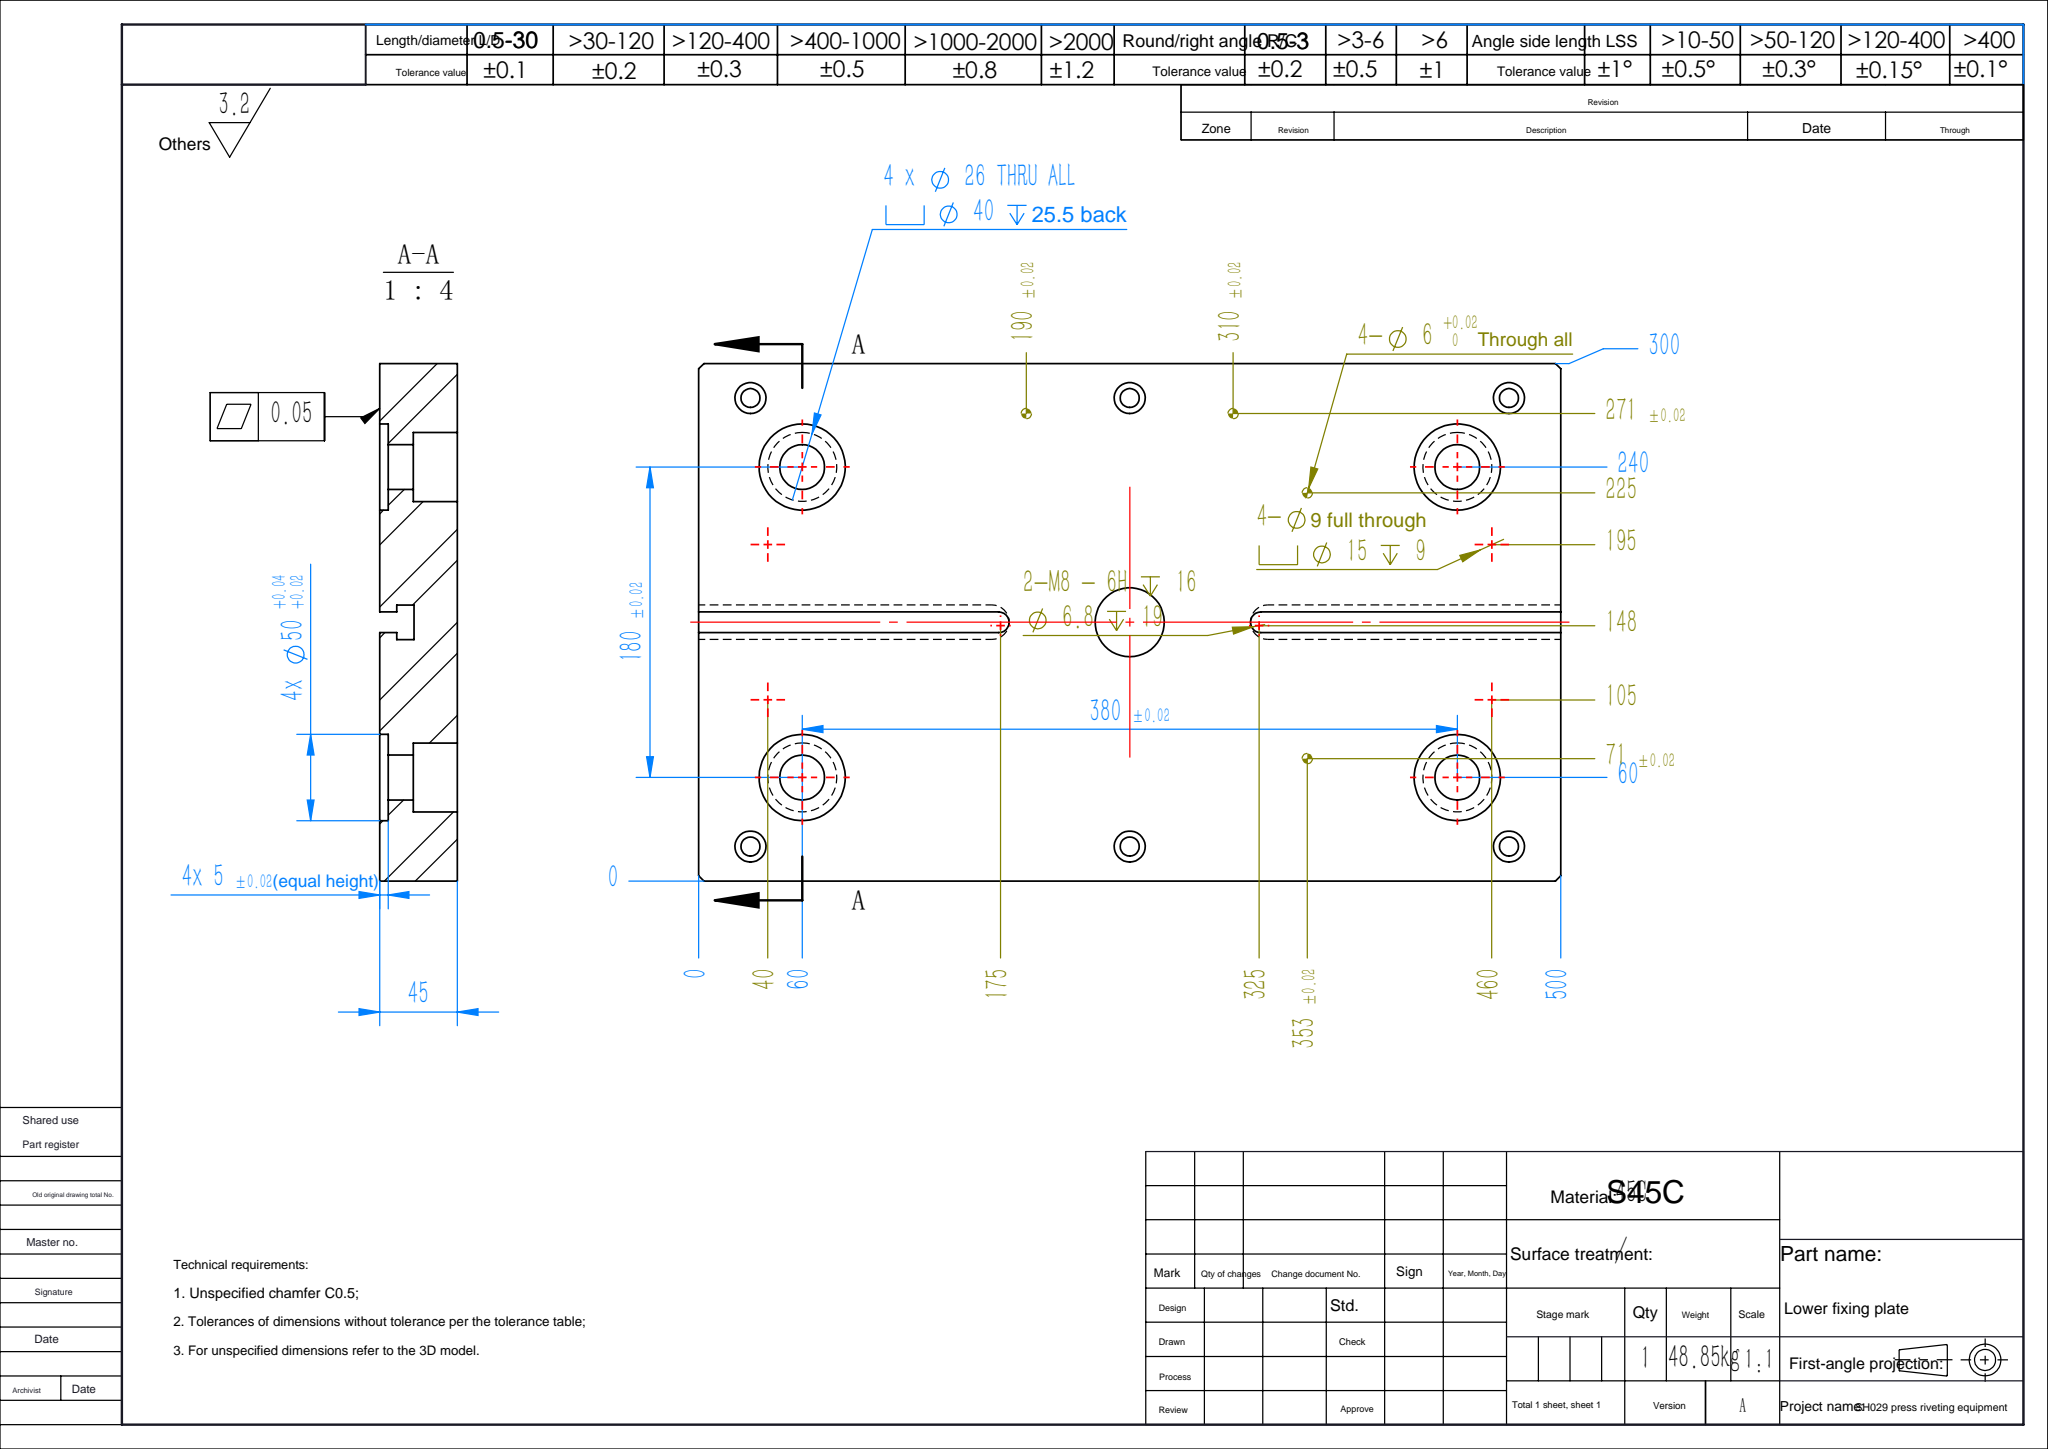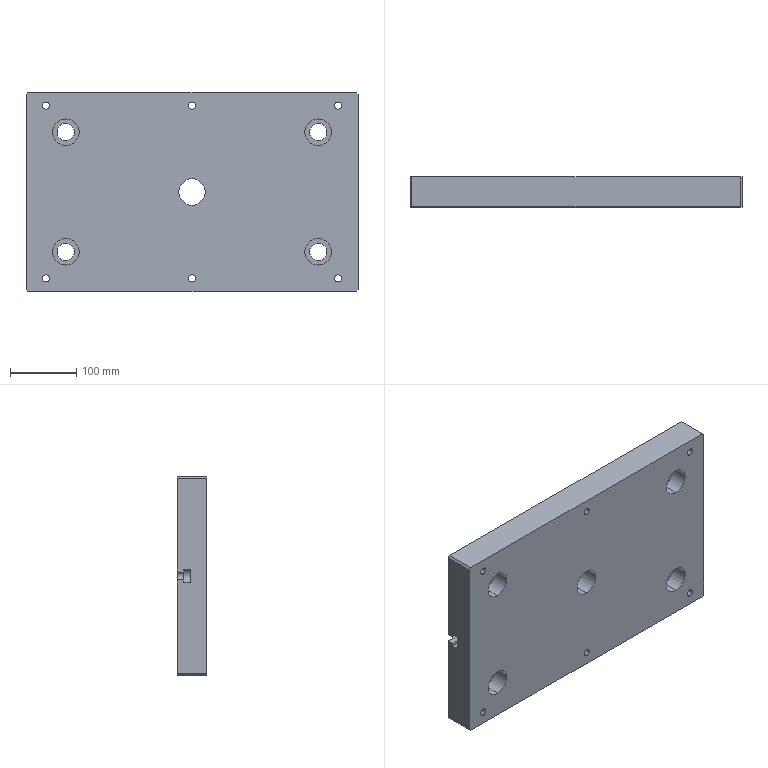Part | SolidWorks | features ICE 3, Fillet 2, HoleWzd 2, Chamfer 1, Extrusion 1, MirrorPattern 1 | 1 solid | 92 faces | box 500 x 45 x 300 mm | volume 6344186 mm3 | cylinder 54 | plane 38 | commonest cylinder face diameters 11 x12 18 x12 40 x10 26 x8 50 x8 12 x2